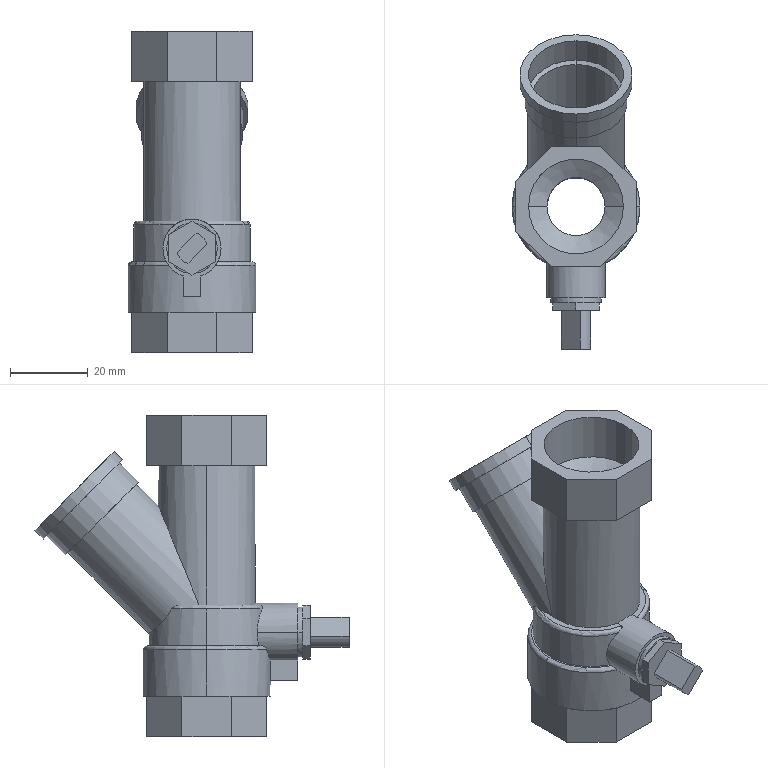Part | SolidWorks | features ICE 13, HoleWzd 3, 3DProfileFeature 2, Extrusion 1, Fillet 1, Sweep 1 | 1 solid | 111 faces | box 33 x 81.096 x 83 mm | volume 34631 mm3 | plane 68 | cylinder 31 | cone 6 | torus 6 | commonest cylinder face diameters 15 x6 24.5 x6 25 x4 30 x3 8 x2 13 x2